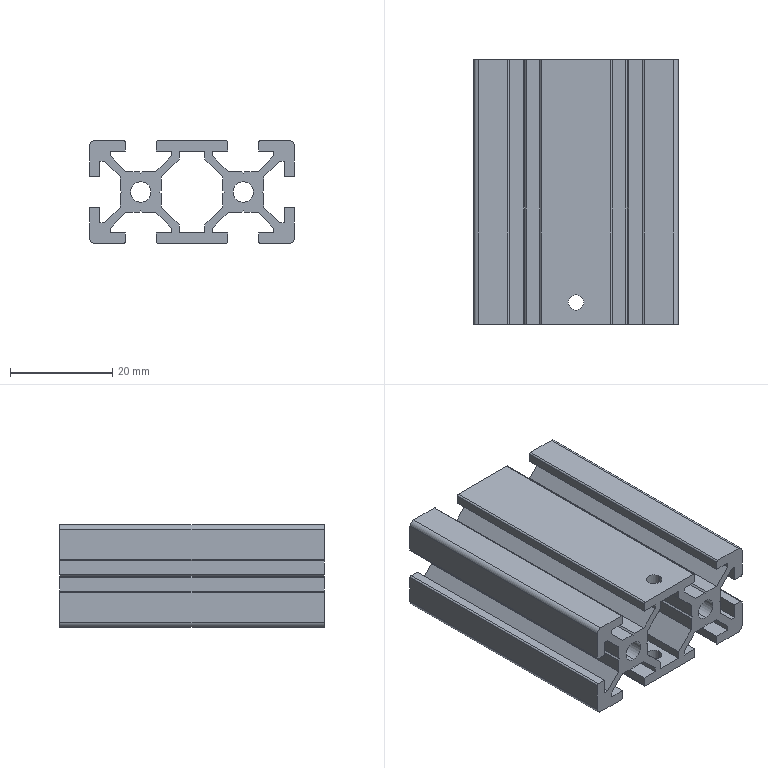Part | SolidWorks | features SplitBody 1 | 1 solid | 126 faces | box 40 x 51.64 x 20 mm | volume 16683 mm3 | plane 102 | cylinder 24 | commonest cylinder face diameters 0.6 x12 2 x4 3 x4 4 x4